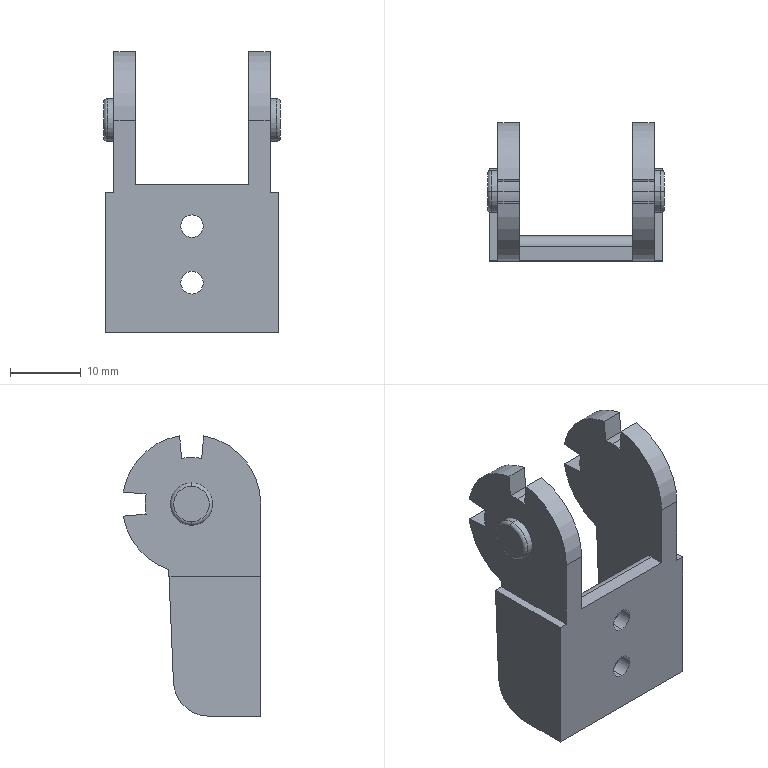Part | STEP file | _VED02-F15-002.stp | 1 solid | 55 faces | box 25 x 19.467 x 39.663 mm | volume 5123 mm3 | plane 24 | cylinder 23 | cone 4 | torus 4 | commonest cylinder face diameters 13.178 x6 3.2 x4 6 x4 19.618 x4 10 x2 19.616 x2